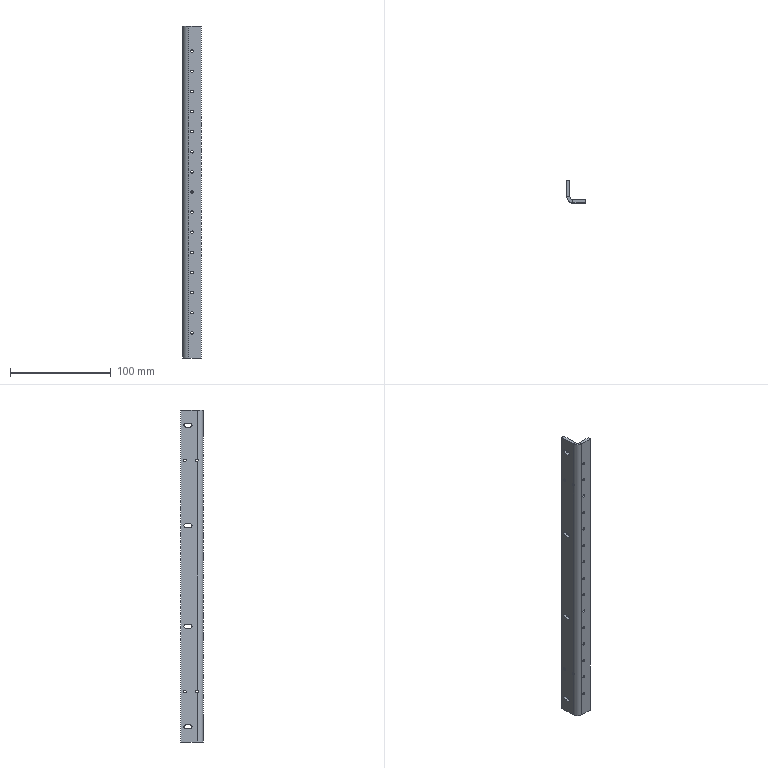Part | STEP file | Guide rail bracket V1.201001 | 1 solid | 72 faces | box 18 x 22 x 330 mm | volume 34095 mm3 | cylinder 52 | plane 20 | commonest cylinder face diameters 2.5 x38 4 x12 6 x1 12 x1